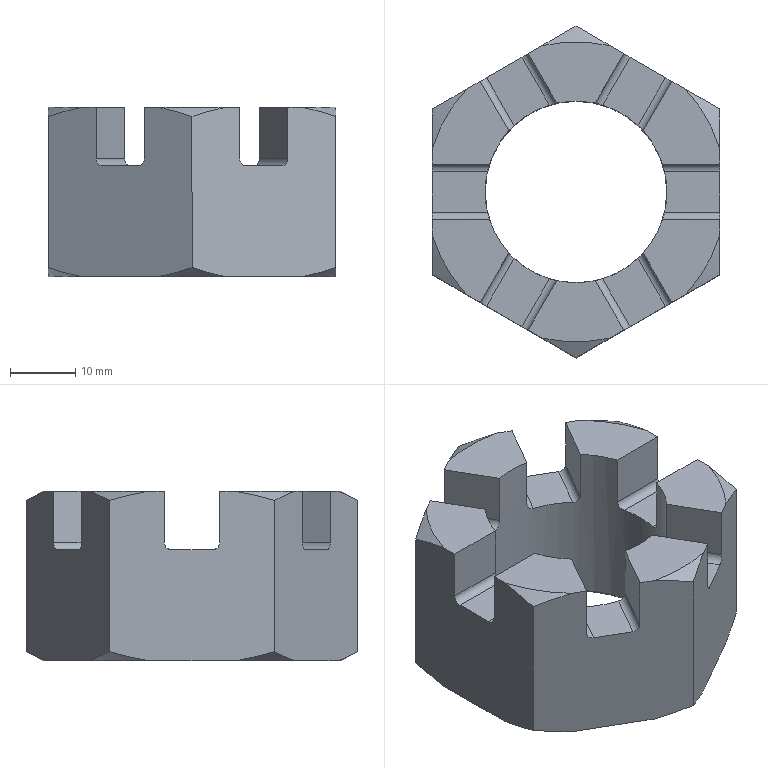Part | SolidWorks | features Cut 3, Chamfer 1, CirPattern 1, Extrusion 1 | 1 solid | 59 faces | box 44.037 x 50.85 x 26 mm | volume 23981 mm3 | plane 31 | cone 14 | cylinder 14 | commonest cylinder face diameters 2.25 x12 27.835 x2